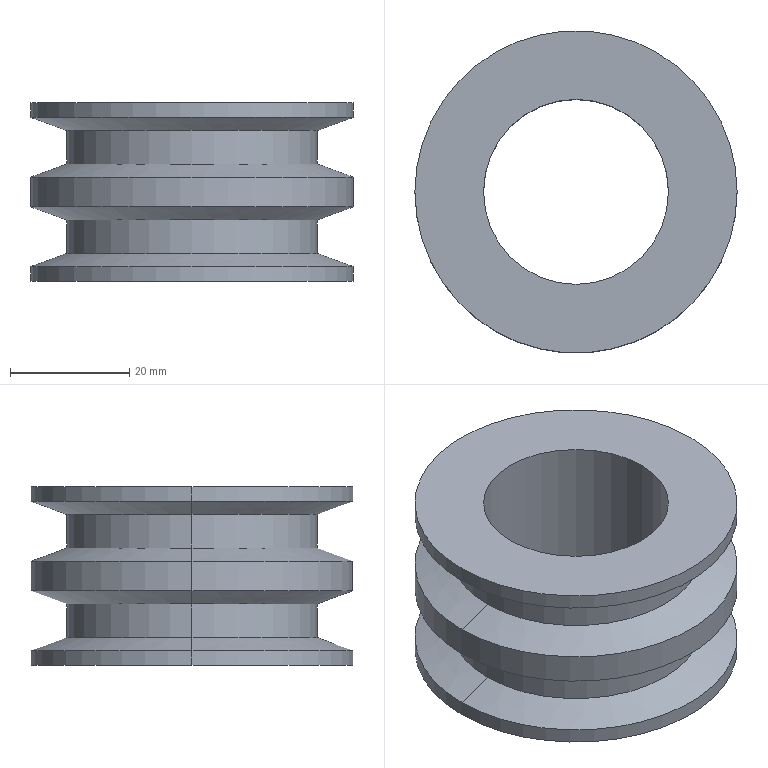Part | SolidWorks | features Extrusion 1, RevCut 1 | 1 solid | 22 faces | box 54 x 54 x 30 mm | volume 31755 mm3 | cylinder 12 | cone 8 | plane 2 | commonest cylinder face diameters 54 x6 42 x4 31 x2
STEP:
#1=CARTESIAN_POINT('',(-27.,0.,2.5));
#2=VERTEX_POINT('',#1);
#3=CARTESIAN_POINT('',(27.,0.,2.5));
#4=VERTEX_POINT('',#3);
#5=CARTESIAN_POINT('',(0.,0.,2.5));
#6=DIRECTION('',(0.,0.,-1.));
#7=DIRECTION('',(-1.,0.,0.));
#8=AXIS2_PLACEMENT_3D('',#5,#6,#7);
#9=CIRCLE('',#8,27.);
#10=EDGE_CURVE('',#2,#4,#9,.T.);
#11=ORIENTED_EDGE('',*,*,#10,.T.);
#12=CARTESIAN_POINT('',(27.,0.,-2.5));
#13=VERTEX_POINT('',#12);
#14=CARTESIAN_POINT('',(27.,0.,15.));
#15=DIRECTION('',(0.,0.,-1.));
#16=VECTOR('',#15,1000.);
#17=LINE('',#14,#16);
#18=EDGE_CURVE('',#4,#13,#17,.T.);
#19=ORIENTED_EDGE('',*,*,#18,.T.);
#20=CARTESIAN_POINT('',(-27.,0.,-2.5));
#21=VERTEX_POINT('',#20);
#22=CARTESIAN_POINT('',(0.,0.,-2.5));
#23=DIRECTION('',(0.,0.,-1.));
#24=DIRECTION('',(-1.,0.,0.));
#25=AXIS2_PLACEMENT_3D('',#22,#23,#24);
#26=CIRCLE('',#25,27.);
#27=EDGE_CURVE('',#21,#13,#26,.T.);
#28=ORIENTED_EDGE('',*,*,#27,.F.);
#29=CARTESIAN_POINT('',(-27.,0.,15.));
#30=DIRECTION('',(0.,0.,-1.));
#31=VECTOR('',#30,1000.);
#32=LINE('',#29,#31);
#33=EDGE_CURVE('',#2,#21,#32,.T.);
#34=ORIENTED_EDGE('',*,*,#33,.F.);
#35=EDGE_LOOP('',(#11,#19,#28,#34));
#36=FACE_OUTER_BOUND('',#35,.T.);
#37=CARTESIAN_POINT('',(0.,0.,15.));
#38=DIRECTION('',(0.,0.,-1.));
#39=DIRECTION('',(-1.,0.,0.));
#40=AXIS2_PLACEMENT_3D('',#37,#38,#39);
#41=CYLINDRICAL_SURFACE('',#40,27.);
#42=ADVANCED_FACE('',(#36),#41,.T.);
#43=CARTESIAN_POINT('',(-21.,0.,10.316));
#44=VERTEX_POINT('',#43);
#45=CARTESIAN_POINT('',(21.,0.,10.316));
#46=VERTEX_POINT('',#45);
#47=CARTESIAN_POINT('',(0.,0.,10.316));
#48=DIRECTION('',(0.,0.,-1.));
#49=DIRECTION('',(-1.,0.,0.));
#50=AXIS2_PLACEMENT_3D('',#47,#48,#49);
#51=CIRCLE('',#50,21.);
#52=EDGE_CURVE('',#44,#46,#51,.T.);
#53=ORIENTED_EDGE('',*,*,#52,.T.);
#54=CARTESIAN_POINT('',(21.,0.,4.684));
#55=VERTEX_POINT('',#54);
#56=CARTESIAN_POINT('',(21.,0.,-19.219));
#57=DIRECTION('',(0.,0.,-1.));
#58=VECTOR('',#57,1000.);
#59=LINE('',#56,#58);
#60=EDGE_CURVE('',#46,#55,#59,.T.);
#61=ORIENTED_EDGE('',*,*,#60,.T.);
#62=CARTESIAN_POINT('',(-21.,0.,4.684));
#63=VERTEX_POINT('',#62);
#64=CARTESIAN_POINT('',(0.,0.,4.684));
#65=DIRECTION('',(0.,0.,-1.));
#66=DIRECTION('',(-1.,0.,0.));
#67=AXIS2_PLACEMENT_3D('',#64,#65,#66);
#68=CIRCLE('',#67,21.);
#69=EDGE_CURVE('',#63,#55,#68,.T.);
#70=ORIENTED_EDGE('',*,*,#69,.F.);
#71=CARTESIAN_POINT('',(-21.,0.,-19.219));
#72=DIRECTION('',(0.,0.,-1.));
#73=VECTOR('',#72,1000.);
#74=LINE('',#71,#73);
#75=EDGE_CURVE('',#44,#63,#74,.T.);
#76=ORIENTED_EDGE('',*,*,#75,.F.);
#77=EDGE_LOOP('',(#53,#61,#70,#76));
#78=FACE_OUTER_BOUND('',#77,.T.);
#79=CARTESIAN_POINT('',(0.,0.,-19.219));
#80=DIRECTION('',(0.,0.,-1.));
#81=DIRECTION('',(-1.,0.,0.));
#82=AXIS2_PLACEMENT_3D('',#79,#80,#81);
#83=CYLINDRICAL_SURFACE('',#82,21.);
#84=ADVANCED_FACE('',(#78),#83,.T.);
#85=ORIENTED_EDGE('',*,*,#69,.T.);
#86=CARTESIAN_POINT('',(21.,0.,4.684));
#87=DIRECTION('',(0.9397,0.,-0.342));
#88=VECTOR('',#87,1000.);
#89=LINE('',#86,#88);
#90=EDGE_CURVE('',#55,#4,#89,.T.);
#91=ORIENTED_EDGE('',*,*,#90,.T.);
#92=ORIENTED_EDGE('',*,*,#10,.F.);
#93=CARTESIAN_POINT('',(-21.,0.,4.684));
#94=DIRECTION('',(-0.9397,0.,-0.342));
#95=VECTOR('',#94,1000.);
#96=LINE('',#93,#95);
#97=EDGE_CURVE('',#63,#2,#96,.T.);
#98=ORIENTED_EDGE('',*,*,#97,.F.);
#99=EDGE_LOOP('',(#85,#91,#92,#98));
#100=FACE_OUTER_BOUND('',#99,.T.);
#101=CARTESIAN_POINT('',(0.,0.,4.684));
#102=DIRECTION('',(0.,0.,-1.));
#103=DIRECTION('',(-1.,0.,0.));
#104=AXIS2_PLACEMENT_3D('',#101,#102,#103);
#105=CONICAL_SURFACE('',#104,21.,1.222);
#106=ADVANCED_FACE('',(#100),#105,.T.);
#107=ORIENTED_EDGE('',*,*,#52,.F.);
#108=CARTESIAN_POINT('',(-27.,0.,12.5));
#109=VERTEX_POINT('',#108);
#110=CARTESIAN_POINT('',(-27.,0.,12.5));
#111=DIRECTION('',(-0.9397,0.,0.342));
#112=VECTOR('',#111,1000.);
#113=LINE('',#110,#112);
#114=EDGE_CURVE('',#44,#109,#113,.T.);
#115=ORIENTED_EDGE('',*,*,#114,.T.);
#116=CARTESIAN_POINT('',(27.,0.,12.5));
#117=VERTEX_POINT('',#116);
#118=CARTESIAN_POINT('',(0.,0.,12.5));
#119=DIRECTION('',(0.,0.,-1.));
#120=DIRECTION('',(-1.,0.,0.));
#121=AXIS2_PLACEMENT_3D('',#118,#119,#120);
#122=CIRCLE('',#121,27.);
#123=EDGE_CURVE('',#109,#117,#122,.T.);
#124=ORIENTED_EDGE('',*,*,#123,.T.);
#125=CARTESIAN_POINT('',(27.,0.,12.5));
#126=DIRECTION('',(0.9397,0.,0.342));
#127=VECTOR('',#126,1000.);
#128=LINE('',#125,#127);
#129=EDGE_CURVE('',#46,#117,#128,.T.);
#130=ORIENTED_EDGE('',*,*,#129,.F.);
#131=EDGE_LOOP('',(#107,#115,#124,#130));
#132=FACE_OUTER_BOUND('',#131,.T.);
#133=CARTESIAN_POINT('',(0.,0.,12.5));
#134=DIRECTION('',(0.,0.,1.));
#135=DIRECTION('',(1.,0.,0.));
#136=AXIS2_PLACEMENT_3D('',#133,#134,#135);
#137=CONICAL_SURFACE('',#136,27.,1.222);
#138=ADVANCED_FACE('',(#132),#137,.T.);
#139=CARTESIAN_POINT('',(-21.,0.,-4.684));
#140=VERTEX_POINT('',#139);
#141=CARTESIAN_POINT('',(21.,0.,-4.684));
#142=VERTEX_POINT('',#141);
#143=CARTESIAN_POINT('',(0.,0.,-4.684));
#144=DIRECTION('',(0.,0.,-1.));
#145=DIRECTION('',(-1.,0.,0.));
#146=AXIS2_PLACEMENT_3D('',#143,#144,#145);
#147=CIRCLE('',#146,21.);
#148=EDGE_CURVE('',#140,#142,#147,.T.);
#149=ORIENTED_EDGE('',*,*,#148,.F.);
#150=CARTESIAN_POINT('',(-27.,0.,-2.5));
#151=DIRECTION('',(-0.9397,0.,0.342));
#152=VECTOR('',#151,1000.);
#153=LINE('',#150,#152);
#154=EDGE_CURVE('',#140,#21,#153,.T.);
#155=ORIENTED_EDGE('',*,*,#154,.T.);
#156=ORIENTED_EDGE('',*,*,#27,.T.);
#157=CARTESIAN_POINT('',(27.,0.,-2.5));
#158=DIRECTION('',(0.9397,0.,0.342));
#159=VECTOR('',#158,1000.);
#160=LINE('',#157,#159);
#161=EDGE_CURVE('',#142,#13,#160,.T.);
#162=ORIENTED_EDGE('',*,*,#161,.F.);
#163=EDGE_LOOP('',(#149,#155,#156,#162));
#164=FACE_OUTER_BOUND('',#163,.T.);
#165=CARTESIAN_POINT('',(0.,0.,-2.5));
#166=DIRECTION('',(0.,0.,1.));
#167=DIRECTION('',(1.,0.,0.));
#168=AXIS2_PLACEMENT_3D('',#165,#166,#167);
#169=CONICAL_SURFACE('',#168,27.,1.222);
#170=ADVANCED_FACE('',(#164),#169,.T.);
#171=ORIENTED_EDGE('',*,*,#148,.T.);
#172=CARTESIAN_POINT('',(21.,0.,-10.316));
#173=VERTEX_POINT('',#172);
#174=CARTESIAN_POINT('',(21.,0.,-19.219));
#175=DIRECTION('',(0.,0.,-1.));
#176=VECTOR('',#175,1000.);
#177=LINE('',#174,#176);
#178=EDGE_CURVE('',#142,#173,#177,.T.);
#179=ORIENTED_EDGE('',*,*,#178,.T.);
#180=CARTESIAN_POINT('',(-21.,0.,-10.316));
#181=VERTEX_POINT('',#180);
#182=CARTESIAN_POINT('',(0.,0.,-10.316));
#183=DIRECTION('',(0.,0.,-1.));
#184=DIRECTION('',(-1.,0.,0.));
#185=AXIS2_PLACEMENT_3D('',#182,#183,#184);
#186=CIRCLE('',#185,21.);
#187=EDGE_CURVE('',#181,#173,#186,.T.);
#188=ORIENTED_EDGE('',*,*,#187,.F.);
#189=CARTESIAN_POINT('',(-21.,0.,-19.219));
#190=DIRECTION('',(0.,0.,-1.));
#191=VECTOR('',#190,1000.);
#192=LINE('',#189,#191);
#193=EDGE_CURVE('',#140,#181,#192,.T.);
#194=ORIENTED_EDGE('',*,*,#193,.F.);
#195=EDGE_LOOP('',(#171,#179,#188,#194));
#196=FACE_OUTER_BOUND('',#195,.T.);
#197=CARTESIAN_POINT('',(0.,0.,-19.219));
#198=DIRECTION('',(0.,0.,-1.));
#199=DIRECTION('',(-1.,0.,0.));
#200=AXIS2_PLACEMENT_3D('',#197,#198,#199);
#201=CYLINDRICAL_SURFACE('',#200,21.);
#202=ADVANCED_FACE('',(#196),#201,.T.);
#203=ORIENTED_EDGE('',*,*,#187,.T.);
#204=CARTESIAN_POINT('',(27.,0.,-12.5));
#205=VERTEX_POINT('',#204);
#206=CARTESIAN_POINT('',(21.,0.,-10.316));
#207=DIRECTION('',(0.9397,0.,-0.342));
#208=VECTOR('',#207,1000.);
#209=LINE('',#206,#208);
#210=EDGE_CURVE('',#173,#205,#209,.T.);
#211=ORIENTED_EDGE('',*,*,#210,.T.);
#212=CARTESIAN_POINT('',(-27.,0.,-12.5));
#213=VERTEX_POINT('',#212);
#214=CARTESIAN_POINT('',(0.,0.,-12.5));
#215=DIRECTION('',(0.,0.,-1.));
#216=DIRECTION('',(-1.,0.,0.));
#217=AXIS2_PLACEMENT_3D('',#214,#215,#216);
#218=CIRCLE('',#217,27.);
#219=EDGE_CURVE('',#213,#205,#218,.T.);
#220=ORIENTED_EDGE('',*,*,#219,.F.);
#221=CARTESIAN_POINT('',(-21.,0.,-10.316));
#222=DIRECTION('',(-0.9397,0.,-0.342));
#223=VECTOR('',#222,1000.);
#224=LINE('',#221,#223);
#225=EDGE_CURVE('',#181,#213,#224,.T.);
#226=ORIENTED_EDGE('',*,*,#225,.F.);
#227=EDGE_LOOP('',(#203,#211,#220,#226));
#228=FACE_OUTER_BOUND('',#227,.T.);
#229=CARTESIAN_POINT('',(0.,0.,-10.316));
#230=DIRECTION('',(0.,0.,-1.));
#231=DIRECTION('',(-1.,0.,0.));
#232=AXIS2_PLACEMENT_3D('',#229,#230,#231);
#233=CONICAL_SURFACE('',#232,21.,1.222);
#234=ADVANCED_FACE('',(#228),#233,.T.);
#235=CARTESIAN_POINT('',(-15.5,0.,15.));
#236=VERTEX_POINT('',#235);
#237=CARTESIAN_POINT('',(15.5,0.,15.));
#238=VERTEX_POINT('',#237);
#239=CARTESIAN_POINT('',(0.,0.,15.));
#240=DIRECTION('',(0.,0.,1.));
#241=DIRECTION('',(1.,0.,0.));
#242=AXIS2_PLACEMENT_3D('',#239,#240,#241);
#243=CIRCLE('',#242,15.5);
#244=EDGE_CURVE('',#236,#238,#243,.T.);
#245=ORIENTED_EDGE('',*,*,#244,.T.);
#246=CARTESIAN_POINT('',(15.5,0.,-15.));
#247=VERTEX_POINT('',#246);
#248=CARTESIAN_POINT('',(15.5,0.,15.));
#249=DIRECTION('',(0.,0.,-1.));
#250=VECTOR('',#249,1000.);
#251=LINE('',#248,#250);
#252=EDGE_CURVE('',#238,#247,#251,.T.);
#253=ORIENTED_EDGE('',*,*,#252,.T.);
#254=CARTESIAN_POINT('',(-15.5,0.,-15.));
#255=VERTEX_POINT('',#254);
#256=CARTESIAN_POINT('',(0.,0.,-15.));
#257=DIRECTION('',(0.,0.,1.));
#258=DIRECTION('',(1.,0.,0.));
#259=AXIS2_PLACEMENT_3D('',#256,#257,#258);
#260=CIRCLE('',#259,15.5);
#261=EDGE_CURVE('',#255,#247,#260,.T.);
#262=ORIENTED_EDGE('',*,*,#261,.F.);
#263=CARTESIAN_POINT('',(-15.5,0.,15.));
#264=DIRECTION('',(0.,0.,-1.));
#265=VECTOR('',#264,1000.);
#266=LINE('',#263,#265);
#267=EDGE_CURVE('',#236,#255,#266,.T.);
#268=ORIENTED_EDGE('',*,*,#267,.F.);
#269=EDGE_LOOP('',(#245,#253,#262,#268));
#270=FACE_OUTER_BOUND('',#269,.T.);
#271=CARTESIAN_POINT('',(0.,0.,15.));
#272=DIRECTION('',(0.,0.,-1.));
#273=DIRECTION('',(-1.,0.,0.));
#274=AXIS2_PLACEMENT_3D('',#271,#272,#273);
#275=CYLINDRICAL_SURFACE('',#274,15.5);
#276=ADVANCED_FACE('',(#270),#275,.F.);
#277=ORIENTED_EDGE('',*,*,#219,.T.);
#278=CARTESIAN_POINT('',(27.,0.,-15.));
#279=VERTEX_POINT('',#278);
#280=CARTESIAN_POINT('',(27.,0.,15.));
#281=DIRECTION('',(0.,0.,-1.));
#282=VECTOR('',#281,1000.);
#283=LINE('',#280,#282);
#284=EDGE_CURVE('',#205,#279,#283,.T.);
#285=ORIENTED_EDGE('',*,*,#284,.T.);
#286=CARTESIAN_POINT('',(-27.,0.,-15.));
#287=VERTEX_POINT('',#286);
#288=CARTESIAN_POINT('',(0.,0.,-15.));
#289=DIRECTION('',(0.,0.,1.));
#290=DIRECTION('',(1.,0.,0.));
#291=AXIS2_PLACEMENT_3D('',#288,#289,#290);
#292=CIRCLE('',#291,27.);
#293=EDGE_CURVE('',#279,#287,#292,.T.);
#294=ORIENTED_EDGE('',*,*,#293,.T.);
#295=CARTESIAN_POINT('',(-27.,0.,15.));
#296=DIRECTION('',(0.,0.,-1.));
#297=VECTOR('',#296,1000.);
#298=LINE('',#295,#297);
#299=EDGE_CURVE('',#213,#287,#298,.T.);
#300=ORIENTED_EDGE('',*,*,#299,.F.);
#301=EDGE_LOOP('',(#277,#285,#294,#300));
#302=FACE_OUTER_BOUND('',#301,.T.);
#303=CARTESIAN_POINT('',(0.,0.,15.));
#304=DIRECTION('',(0.,0.,-1.));
#305=DIRECTION('',(-1.,0.,0.));
#306=AXIS2_PLACEMENT_3D('',#303,#304,#305);
#307=CYLINDRICAL_SURFACE('',#306,27.);
#308=ADVANCED_FACE('',(#302),#307,.T.);
#309=CARTESIAN_POINT('',(27.,0.,15.));
#310=VERTEX_POINT('',#309);
#311=CARTESIAN_POINT('',(-27.,0.,15.));
#312=VERTEX_POINT('',#311);
#313=CARTESIAN_POINT('',(0.,0.,15.));
#314=DIRECTION('',(0.,0.,1.));
#315=DIRECTION('',(1.,0.,0.));
#316=AXIS2_PLACEMENT_3D('',#313,#314,#315);
#317=CIRCLE('',#316,27.);
#318=EDGE_CURVE('',#310,#312,#317,.T.);
#319=ORIENTED_EDGE('',*,*,#318,.F.);
#320=CARTESIAN_POINT('',(27.,0.,15.));
#321=DIRECTION('',(0.,0.,-1.));
#322=VECTOR('',#321,1000.);
#323=LINE('',#320,#322);
#324=EDGE_CURVE('',#310,#117,#323,.T.);
#325=ORIENTED_EDGE('',*,*,#324,.T.);
#326=ORIENTED_EDGE('',*,*,#123,.F.);
#327=CARTESIAN_POINT('',(-27.,0.,15.));
#328=DIRECTION('',(0.,0.,-1.));
#329=VECTOR('',#328,1000.);
#330=LINE('',#327,#329);
#331=EDGE_CURVE('',#312,#109,#330,.T.);
#332=ORIENTED_EDGE('',*,*,#331,.F.);
#333=EDGE_LOOP('',(#319,#325,#326,#332));
#334=FACE_OUTER_BOUND('',#333,.T.);
#335=CARTESIAN_POINT('',(0.,0.,15.));
#336=DIRECTION('',(0.,0.,-1.));
#337=DIRECTION('',(-1.,0.,0.));
#338=AXIS2_PLACEMENT_3D('',#335,#336,#337);
#339=CYLINDRICAL_SURFACE('',#338,27.);
#340=ADVANCED_FACE('',(#334),#339,.T.);
#341=ORIENTED_EDGE('',*,*,#324,.F.);
#342=CARTESIAN_POINT('',(0.,0.,15.));
#343=DIRECTION('',(0.,0.,1.));
#344=DIRECTION('',(1.,0.,0.));
#345=AXIS2_PLACEMENT_3D('',#342,#343,#344);
#346=CIRCLE('',#345,27.);
#347=EDGE_CURVE('',#312,#310,#346,.T.);
#348=ORIENTED_EDGE('',*,*,#347,.F.);
#349=ORIENTED_EDGE('',*,*,#331,.T.);
#350=CARTESIAN_POINT('',(0.,0.,12.5));
#351=DIRECTION('',(0.,0.,-1.));
#352=DIRECTION('',(-1.,0.,0.));
#353=AXIS2_PLACEMENT_3D('',#350,#351,#352);
#354=CIRCLE('',#353,27.);
#355=EDGE_CURVE('',#117,#109,#354,.T.);
#356=ORIENTED_EDGE('',*,*,#355,.F.);
#357=EDGE_LOOP('',(#341,#348,#349,#356));
#358=FACE_OUTER_BOUND('',#357,.T.);
#359=CARTESIAN_POINT('',(0.,0.,15.));
#360=DIRECTION('',(0.,0.,-1.));
#361=DIRECTION('',(-1.,0.,0.));
#362=AXIS2_PLACEMENT_3D('',#359,#360,#361);
#363=CYLINDRICAL_SURFACE('',#362,27.);
#364=ADVANCED_FACE('',(#358),#363,.T.);
#365=ORIENTED_EDGE('',*,*,#284,.F.);
#366=CARTESIAN_POINT('',(0.,0.,-12.5));
#367=DIRECTION('',(0.,0.,-1.));
#368=DIRECTION('',(-1.,0.,0.));
#369=AXIS2_PLACEMENT_3D('',#366,#367,#368);
#370=CIRCLE('',#369,27.);
#371=EDGE_CURVE('',#205,#213,#370,.T.);
#372=ORIENTED_EDGE('',*,*,#371,.T.);
#373=ORIENTED_EDGE('',*,*,#299,.T.);
#374=CARTESIAN_POINT('',(0.,0.,-15.));
#375=DIRECTION('',(0.,0.,1.));
#376=DIRECTION('',(1.,0.,0.));
#377=AXIS2_PLACEMENT_3D('',#374,#375,#376);
#378=CIRCLE('',#377,27.);
#379=EDGE_CURVE('',#287,#279,#378,.T.);
#380=ORIENTED_EDGE('',*,*,#379,.T.);
#381=EDGE_LOOP('',(#365,#372,#373,#380));
#382=FACE_OUTER_BOUND('',#381,.T.);
#383=CARTESIAN_POINT('',(0.,0.,15.));
#384=DIRECTION('',(0.,0.,-1.));
#385=DIRECTION('',(-1.,0.,0.));
#386=AXIS2_PLACEMENT_3D('',#383,#384,#385);
#387=CYLINDRICAL_SURFACE('',#386,27.);
#388=ADVANCED_FACE('',(#382),#387,.T.);
#389=ORIENTED_EDGE('',*,*,#347,.T.);
#390=ORIENTED_EDGE('',*,*,#318,.T.);
#391=EDGE_LOOP('',(#389,#390));
#392=FACE_OUTER_BOUND('',#391,.T.);
#393=ORIENTED_EDGE('',*,*,#244,.F.);
#394=CARTESIAN_POINT('',(0.,0.,15.));
#395=DIRECTION('',(0.,0.,1.));
#396=DIRECTION('',(1.,0.,0.));
#397=AXIS2_PLACEMENT_3D('',#394,#395,#396);
#398=CIRCLE('',#397,15.5);
#399=EDGE_CURVE('',#238,#236,#398,.T.);
#400=ORIENTED_EDGE('',*,*,#399,.F.);
#401=EDGE_LOOP('',(#393,#400));
#402=FACE_BOUND('',#401,.T.);
#403=CARTESIAN_POINT('',(0.,0.,15.));
#404=DIRECTION('',(0.,0.,1.));
#405=DIRECTION('',(1.,0.,0.));
#406=AXIS2_PLACEMENT_3D('',#403,#404,#405);
#407=PLANE('',#406);
#408=ADVANCED_FACE('',(#392,#402),#407,.T.);
#409=ORIENTED_EDGE('',*,*,#379,.F.);
#410=ORIENTED_EDGE('',*,*,#293,.F.);
#411=EDGE_LOOP('',(#409,#410));
#412=FACE_OUTER_BOUND('',#411,.T.);
#413=ORIENTED_EDGE('',*,*,#261,.T.);
#414=CARTESIAN_POINT('',(0.,0.,-15.));
#415=DIRECTION('',(0.,0.,1.));
#416=DIRECTION('',(1.,0.,0.));
#417=AXIS2_PLACEMENT_3D('',#414,#415,#416);
#418=CIRCLE('',#417,15.5);
#419=EDGE_CURVE('',#247,#255,#418,.T.);
#420=ORIENTED_EDGE('',*,*,#419,.T.);
#421=EDGE_LOOP('',(#413,#420));
#422=FACE_BOUND('',#421,.T.);
#423=CARTESIAN_POINT('',(0.,0.,-15.));
#424=DIRECTION('',(0.,0.,1.));
#425=DIRECTION('',(1.,0.,0.));
#426=AXIS2_PLACEMENT_3D('',#423,#424,#425);
#427=PLANE('',#426);
#428=ADVANCED_FACE('',(#412,#422),#427,.F.);
#429=ORIENTED_EDGE('',*,*,#252,.F.);
#430=ORIENTED_EDGE('',*,*,#399,.T.);
#431=ORIENTED_EDGE('',*,*,#267,.T.);
#432=ORIENTED_EDGE('',*,*,#419,.F.);
#433=EDGE_LOOP('',(#429,#430,#431,#432));
#434=FACE_OUTER_BOUND('',#433,.T.);
#435=CARTESIAN_POINT('',(0.,0.,15.));
#436=DIRECTION('',(0.,0.,-1.));
#437=DIRECTION('',(-1.,0.,0.));
#438=AXIS2_PLACEMENT_3D('',#435,#436,#437);
#439=CYLINDRICAL_SURFACE('',#438,15.5);
#440=ADVANCED_FACE('',(#434),#439,.F.);
#441=ORIENTED_EDGE('',*,*,#210,.F.);
#442=CARTESIAN_POINT('',(0.,0.,-10.316));
#443=DIRECTION('',(0.,0.,-1.));
#444=DIRECTION('',(-1.,0.,0.));
#445=AXIS2_PLACEMENT_3D('',#442,#443,#444);
#446=CIRCLE('',#445,21.);
#447=EDGE_CURVE('',#173,#181,#446,.T.);
#448=ORIENTED_EDGE('',*,*,#447,.T.);
#449=ORIENTED_EDGE('',*,*,#225,.T.);
#450=ORIENTED_EDGE('',*,*,#371,.F.);
#451=EDGE_LOOP('',(#441,#448,#449,#450));
#452=FACE_OUTER_BOUND('',#451,.T.);
#453=CARTESIAN_POINT('',(0.,0.,-10.316));
#454=DIRECTION('',(0.,0.,-1.));
#455=DIRECTION('',(-1.,0.,0.));
#456=AXIS2_PLACEMENT_3D('',#453,#454,#455);
#457=CONICAL_SURFACE('',#456,21.,1.222);
#458=ADVANCED_FACE('',(#452),#457,.T.);
#459=ORIENTED_EDGE('',*,*,#178,.F.);
#460=CARTESIAN_POINT('',(0.,0.,-4.684));
#461=DIRECTION('',(0.,0.,-1.));
#462=DIRECTION('',(-1.,0.,0.));
#463=AXIS2_PLACEMENT_3D('',#460,#461,#462);
#464=CIRCLE('',#463,21.);
#465=EDGE_CURVE('',#142,#140,#464,.T.);
#466=ORIENTED_EDGE('',*,*,#465,.T.);
#467=ORIENTED_EDGE('',*,*,#193,.T.);
#468=ORIENTED_EDGE('',*,*,#447,.F.);
#469=EDGE_LOOP('',(#459,#466,#467,#468));
#470=FACE_OUTER_BOUND('',#469,.T.);
#471=CARTESIAN_POINT('',(0.,0.,-19.219));
#472=DIRECTION('',(0.,0.,-1.));
#473=DIRECTION('',(-1.,0.,0.));
#474=AXIS2_PLACEMENT_3D('',#471,#472,#473);
#475=CYLINDRICAL_SURFACE('',#474,21.);
#476=ADVANCED_FACE('',(#470),#475,.T.);
#477=ORIENTED_EDGE('',*,*,#154,.F.);
#478=ORIENTED_EDGE('',*,*,#465,.F.);
#479=ORIENTED_EDGE('',*,*,#161,.T.);
#480=CARTESIAN_POINT('',(0.,0.,-2.5));
#481=DIRECTION('',(0.,0.,-1.));
#482=DIRECTION('',(-1.,0.,0.));
#483=AXIS2_PLACEMENT_3D('',#480,#481,#482);
#484=CIRCLE('',#483,27.);
#485=EDGE_CURVE('',#13,#21,#484,.T.);
#486=ORIENTED_EDGE('',*,*,#485,.T.);
#487=EDGE_LOOP('',(#477,#478,#479,#486));
#488=FACE_OUTER_BOUND('',#487,.T.);
#489=CARTESIAN_POINT('',(0.,0.,-2.5));
#490=DIRECTION('',(0.,0.,1.));
#491=DIRECTION('',(1.,0.,0.));
#492=AXIS2_PLACEMENT_3D('',#489,#490,#491);
#493=CONICAL_SURFACE('',#492,27.,1.222);
#494=ADVANCED_FACE('',(#488),#493,.T.);
#495=ORIENTED_EDGE('',*,*,#114,.F.);
#496=CARTESIAN_POINT('',(0.,0.,10.316));
#497=DIRECTION('',(0.,0.,-1.));
#498=DIRECTION('',(-1.,0.,0.));
#499=AXIS2_PLACEMENT_3D('',#496,#497,#498);
#500=CIRCLE('',#499,21.);
#501=EDGE_CURVE('',#46,#44,#500,.T.);
#502=ORIENTED_EDGE('',*,*,#501,.F.);
#503=ORIENTED_EDGE('',*,*,#129,.T.);
#504=ORIENTED_EDGE('',*,*,#355,.T.);
#505=EDGE_LOOP('',(#495,#502,#503,#504));
#506=FACE_OUTER_BOUND('',#505,.T.);
#507=CARTESIAN_POINT('',(0.,0.,12.5));
#508=DIRECTION('',(0.,0.,1.));
#509=DIRECTION('',(1.,0.,0.));
#510=AXIS2_PLACEMENT_3D('',#507,#508,#509);
#511=CONICAL_SURFACE('',#510,27.,1.222);
#512=ADVANCED_FACE('',(#506),#511,.T.);
#513=ORIENTED_EDGE('',*,*,#90,.F.);
#514=CARTESIAN_POINT('',(0.,0.,4.684));
#515=DIRECTION('',(0.,0.,-1.));
#516=DIRECTION('',(-1.,0.,0.));
#517=AXIS2_PLACEMENT_3D('',#514,#515,#516);
#518=CIRCLE('',#517,21.);
#519=EDGE_CURVE('',#55,#63,#518,.T.);
#520=ORIENTED_EDGE('',*,*,#519,.T.);
#521=ORIENTED_EDGE('',*,*,#97,.T.);
#522=CARTESIAN_POINT('',(0.,0.,2.5));
#523=DIRECTION('',(0.,0.,-1.));
#524=DIRECTION('',(-1.,0.,0.));
#525=AXIS2_PLACEMENT_3D('',#522,#523,#524);
#526=CIRCLE('',#525,27.);
#527=EDGE_CURVE('',#4,#2,#526,.T.);
#528=ORIENTED_EDGE('',*,*,#527,.F.);
#529=EDGE_LOOP('',(#513,#520,#521,#528));
#530=FACE_OUTER_BOUND('',#529,.T.);
#531=CARTESIAN_POINT('',(0.,0.,4.684));
#532=DIRECTION('',(0.,0.,-1.));
#533=DIRECTION('',(-1.,0.,0.));
#534=AXIS2_PLACEMENT_3D('',#531,#532,#533);
#535=CONICAL_SURFACE('',#534,21.,1.222);
#536=ADVANCED_FACE('',(#530),#535,.T.);
#537=ORIENTED_EDGE('',*,*,#60,.F.);
#538=ORIENTED_EDGE('',*,*,#501,.T.);
#539=ORIENTED_EDGE('',*,*,#75,.T.);
#540=ORIENTED_EDGE('',*,*,#519,.F.);
#541=EDGE_LOOP('',(#537,#538,#539,#540));
#542=FACE_OUTER_BOUND('',#541,.T.);
#543=CARTESIAN_POINT('',(0.,0.,-19.219));
#544=DIRECTION('',(0.,0.,-1.));
#545=DIRECTION('',(-1.,0.,0.));
#546=AXIS2_PLACEMENT_3D('',#543,#544,#545);
#547=CYLINDRICAL_SURFACE('',#546,21.);
#548=ADVANCED_FACE('',(#542),#547,.T.);
#549=ORIENTED_EDGE('',*,*,#18,.F.);
#550=ORIENTED_EDGE('',*,*,#527,.T.);
#551=ORIENTED_EDGE('',*,*,#33,.T.);
#552=ORIENTED_EDGE('',*,*,#485,.F.);
#553=EDGE_LOOP('',(#549,#550,#551,#552));
#554=FACE_OUTER_BOUND('',#553,.T.);
#555=CARTESIAN_POINT('',(0.,0.,15.));
#556=DIRECTION('',(0.,0.,-1.));
#557=DIRECTION('',(-1.,0.,0.));
#558=AXIS2_PLACEMENT_3D('',#555,#556,#557);
#559=CYLINDRICAL_SURFACE('',#558,27.);
#560=ADVANCED_FACE('',(#554),#559,.T.);
#561=CLOSED_SHELL('',(#42,#84,#106,#138,#170,#202,#234,#276,#308,#340,#364,#388,#408,#428,#440,#458,#476,#494,#512,#536,#548,#560));
#562=MANIFOLD_SOLID_BREP('',#561);
#563=CARTESIAN_POINT('',(0.,0.,0.));
#564=DIRECTION('',(0.,0.,1.));
#565=DIRECTION('',(1.,0.,0.));
#566=AXIS2_PLACEMENT_3D('',#563,#564,#565);
#567=(LENGTH_UNIT()NAMED_UNIT(*)SI_UNIT(.MILLI.,.METRE.));
#568=UNCERTAINTY_MEASURE_WITH_UNIT(LENGTH_MEASURE(0.00001),#567,'','');
#569=(NAMED_UNIT(*)PLANE_ANGLE_UNIT()SI_UNIT($,.RADIAN.));
#570=(NAMED_UNIT(*)SI_UNIT($,.STERADIAN.)SOLID_ANGLE_UNIT());
#571=(GEOMETRIC_REPRESENTATION_CONTEXT(3)GLOBAL_UNCERTAINTY_ASSIGNED_CONTEXT((#568))GLOBAL_UNIT_ASSIGNED_CONTEXT((#567,#569,#570))REPRESENTATION_CONTEXT('',''));
#572=ADVANCED_BREP_SHAPE_REPRESENTATION('',(#562,#566),#571);